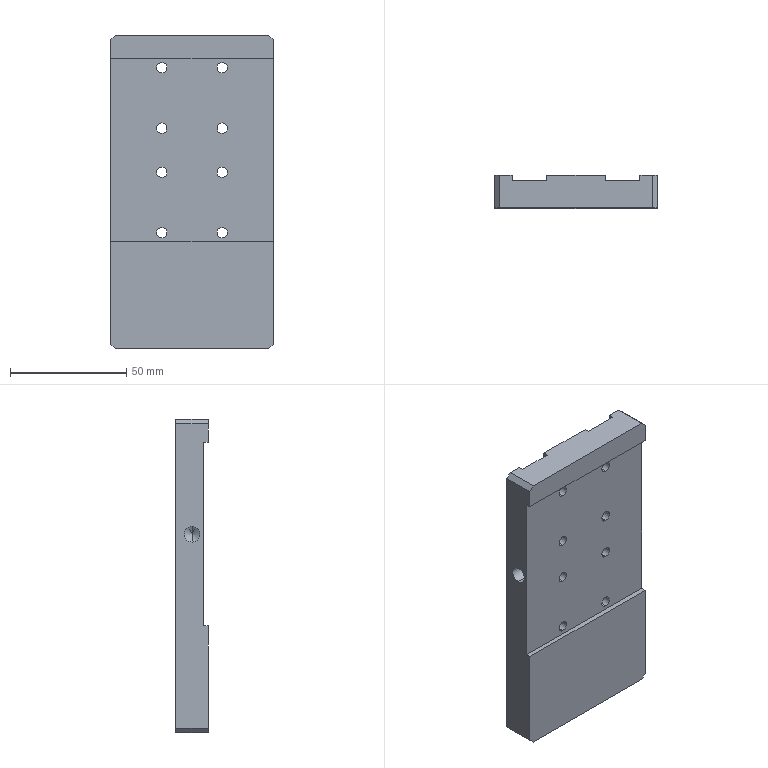Part | STEP file | PN_0043 | 1 solid | 106 faces | box 70 x 14 x 135 mm | volume 108466 mm3 | cylinder 50 | plane 38 | cone 18 | commonest cylinder face diameters 4.5 x16 8 x16 2.5 x12 5 x4 6.8 x2